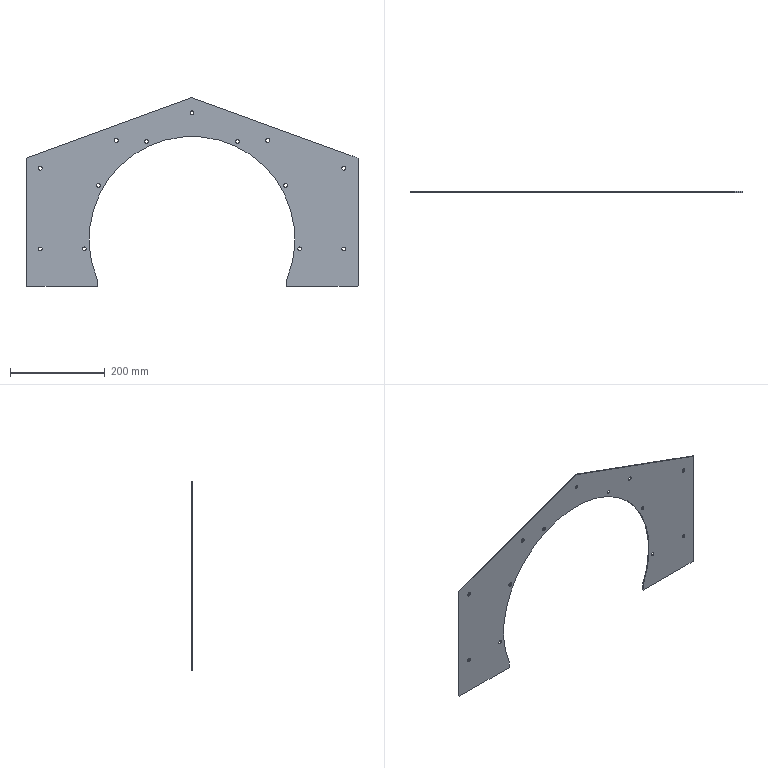Part | NX | features solid 2 | 1 solid | 39 faces | box 700 x 2 x 398 mm | volume 235730 mm3 | cylinder 27 | plane 12 | commonest cylinder face diameters 8 x26 434 x1
STEP:
#1=CARTESIAN_POINT('',(300.,-652.582,589.358));
#2=VERTEX_POINT('',#1);
#3=CARTESIAN_POINT('',(300.,-650.582,589.358));
#4=VERTEX_POINT('',#3);
#5=CARTESIAN_POINT('',(300.,-642.582,589.358));
#6=DIRECTION('',(0.,-1.,0.));
#7=VECTOR('',#6,1000.);
#8=LINE('',#5,#7);
#9=EDGE_CURVE('',#2,#4,#8,.F.);
#10=ORIENTED_EDGE('',*,*,#9,.T.);
#11=CARTESIAN_POINT('',(300.,-650.582,581.358));
#12=VERTEX_POINT('',#11);
#13=CARTESIAN_POINT('',(300.,-650.582,585.358));
#14=DIRECTION('',(0.,1.,0.));
#15=DIRECTION('',(0.,0.,1.));
#16=AXIS2_PLACEMENT_3D('',#13,#14,#15);
#17=CIRCLE('',#16,4.);
#18=EDGE_CURVE('',#4,#12,#17,.T.);
#19=ORIENTED_EDGE('',*,*,#18,.T.);
#20=CARTESIAN_POINT('',(300.,-652.582,581.358));
#21=VERTEX_POINT('',#20);
#22=CARTESIAN_POINT('',(300.,-642.582,581.358));
#23=DIRECTION('',(0.,-1.,0.));
#24=VECTOR('',#23,1000.);
#25=LINE('',#22,#24);
#26=EDGE_CURVE('',#12,#21,#25,.T.);
#27=ORIENTED_EDGE('',*,*,#26,.T.);
#28=CARTESIAN_POINT('',(300.,-652.582,585.358));
#29=DIRECTION('',(0.,-1.,0.));
#30=DIRECTION('',(1.,0.,0.));
#31=AXIS2_PLACEMENT_3D('',#28,#29,#30);
#32=CIRCLE('',#31,4.);
#33=EDGE_CURVE('',#21,#2,#32,.T.);
#34=ORIENTED_EDGE('',*,*,#33,.T.);
#35=EDGE_LOOP('',(#10,#19,#27,#34));
#36=FACE_BOUND('',#35,.T.);
#37=CARTESIAN_POINT('',(300.,-642.582,585.358));
#38=DIRECTION('',(0.,-1.,0.));
#39=DIRECTION('',(0.,0.,-1.));
#40=AXIS2_PLACEMENT_3D('',#37,#38,#39);
#41=CYLINDRICAL_SURFACE('',#40,4.);
#42=ADVANCED_FACE('',(#36),#41,.F.);
#43=CARTESIAN_POINT('',(300.,-650.582,419.358));
#44=VERTEX_POINT('',#43);
#45=CARTESIAN_POINT('',(300.,-652.582,419.358));
#46=VERTEX_POINT('',#45);
#47=CARTESIAN_POINT('',(300.,-642.582,419.358));
#48=DIRECTION('',(0.,-1.,0.));
#49=VECTOR('',#48,1000.);
#50=LINE('',#47,#49);
#51=EDGE_CURVE('',#44,#46,#50,.T.);
#52=ORIENTED_EDGE('',*,*,#51,.F.);
#53=CARTESIAN_POINT('',(300.,-650.582,411.358));
#54=VERTEX_POINT('',#53);
#55=CARTESIAN_POINT('',(300.,-650.582,415.358));
#56=DIRECTION('',(0.,1.,0.));
#57=DIRECTION('',(0.,0.,1.));
#58=AXIS2_PLACEMENT_3D('',#55,#56,#57);
#59=CIRCLE('',#58,4.);
#60=EDGE_CURVE('',#44,#54,#59,.T.);
#61=ORIENTED_EDGE('',*,*,#60,.T.);
#62=CARTESIAN_POINT('',(300.,-652.582,411.358));
#63=VERTEX_POINT('',#62);
#64=CARTESIAN_POINT('',(300.,-642.582,411.358));
#65=DIRECTION('',(0.,-1.,0.));
#66=VECTOR('',#65,1000.);
#67=LINE('',#64,#66);
#68=EDGE_CURVE('',#63,#54,#67,.F.);
#69=ORIENTED_EDGE('',*,*,#68,.F.);
#70=CARTESIAN_POINT('',(300.,-652.582,415.358));
#71=DIRECTION('',(0.,-1.,0.));
#72=DIRECTION('',(1.,0.,0.));
#73=AXIS2_PLACEMENT_3D('',#70,#71,#72);
#74=CIRCLE('',#73,4.);
#75=EDGE_CURVE('',#63,#46,#74,.T.);
#76=ORIENTED_EDGE('',*,*,#75,.T.);
#77=EDGE_LOOP('',(#52,#61,#69,#76));
#78=FACE_BOUND('',#77,.T.);
#79=CARTESIAN_POINT('',(300.,-642.582,415.358));
#80=DIRECTION('',(0.,-1.,0.));
#81=DIRECTION('',(0.,0.,-1.));
#82=AXIS2_PLACEMENT_3D('',#79,#80,#81);
#83=CYLINDRICAL_SURFACE('',#82,4.);
#84=ADVANCED_FACE('',(#78),#83,.F.);
#85=CARTESIAN_POINT('',(207.132,-652.582,419.487));
#86=VERTEX_POINT('',#85);
#87=CARTESIAN_POINT('',(207.132,-650.582,419.487));
#88=VERTEX_POINT('',#87);
#89=CARTESIAN_POINT('',(207.132,-642.582,419.487));
#90=DIRECTION('',(0.,-1.,0.));
#91=VECTOR('',#90,1000.);
#92=LINE('',#89,#91);
#93=EDGE_CURVE('',#86,#88,#92,.F.);
#94=ORIENTED_EDGE('',*,*,#93,.T.);
#95=CARTESIAN_POINT('',(207.132,-650.582,411.487));
#96=VERTEX_POINT('',#95);
#97=CARTESIAN_POINT('',(207.132,-650.582,415.487));
#98=DIRECTION('',(0.,1.,0.));
#99=DIRECTION('',(0.,0.,1.));
#100=AXIS2_PLACEMENT_3D('',#97,#98,#99);
#101=CIRCLE('',#100,4.);
#102=EDGE_CURVE('',#88,#96,#101,.T.);
#103=ORIENTED_EDGE('',*,*,#102,.T.);
#104=CARTESIAN_POINT('',(207.132,-652.582,411.487));
#105=VERTEX_POINT('',#104);
#106=CARTESIAN_POINT('',(207.132,-642.582,411.487));
#107=DIRECTION('',(0.,-1.,0.));
#108=VECTOR('',#107,1000.);
#109=LINE('',#106,#108);
#110=EDGE_CURVE('',#96,#105,#109,.T.);
#111=ORIENTED_EDGE('',*,*,#110,.T.);
#112=CARTESIAN_POINT('',(207.132,-652.582,415.487));
#113=DIRECTION('',(0.,-1.,0.));
#114=DIRECTION('',(1.,0.,0.));
#115=AXIS2_PLACEMENT_3D('',#112,#113,#114);
#116=CIRCLE('',#115,4.);
#117=EDGE_CURVE('',#105,#86,#116,.T.);
#118=ORIENTED_EDGE('',*,*,#117,.T.);
#119=EDGE_LOOP('',(#94,#103,#111,#118));
#120=FACE_BOUND('',#119,.T.);
#121=CARTESIAN_POINT('',(207.132,-642.582,415.487));
#122=DIRECTION('',(0.,-1.,0.));
#123=DIRECTION('',(0.,0.,-1.));
#124=AXIS2_PLACEMENT_3D('',#121,#122,#123);
#125=CYLINDRICAL_SURFACE('',#124,4.);
#126=ADVANCED_FACE('',(#120),#125,.F.);
#127=CARTESIAN_POINT('',(177.334,-650.582,553.289));
#128=VERTEX_POINT('',#127);
#129=CARTESIAN_POINT('',(177.334,-652.582,553.289));
#130=VERTEX_POINT('',#129);
#131=CARTESIAN_POINT('',(177.334,-642.582,553.289));
#132=DIRECTION('',(0.,-1.,0.));
#133=VECTOR('',#132,1000.);
#134=LINE('',#131,#133);
#135=EDGE_CURVE('',#128,#130,#134,.T.);
#136=ORIENTED_EDGE('',*,*,#135,.F.);
#137=CARTESIAN_POINT('',(177.334,-650.582,545.289));
#138=VERTEX_POINT('',#137);
#139=CARTESIAN_POINT('',(177.334,-650.582,549.289));
#140=DIRECTION('',(0.,1.,0.));
#141=DIRECTION('',(0.,0.,1.));
#142=AXIS2_PLACEMENT_3D('',#139,#140,#141);
#143=CIRCLE('',#142,4.);
#144=EDGE_CURVE('',#128,#138,#143,.T.);
#145=ORIENTED_EDGE('',*,*,#144,.T.);
#146=CARTESIAN_POINT('',(177.334,-652.582,545.289));
#147=VERTEX_POINT('',#146);
#148=CARTESIAN_POINT('',(177.334,-642.582,545.289));
#149=DIRECTION('',(0.,-1.,0.));
#150=VECTOR('',#149,1000.);
#151=LINE('',#148,#150);
#152=EDGE_CURVE('',#147,#138,#151,.F.);
#153=ORIENTED_EDGE('',*,*,#152,.F.);
#154=CARTESIAN_POINT('',(177.334,-652.582,549.289));
#155=DIRECTION('',(0.,-1.,0.));
#156=DIRECTION('',(1.,0.,0.));
#157=AXIS2_PLACEMENT_3D('',#154,#155,#156);
#158=CIRCLE('',#157,4.);
#159=EDGE_CURVE('',#147,#130,#158,.T.);
#160=ORIENTED_EDGE('',*,*,#159,.T.);
#161=EDGE_LOOP('',(#136,#145,#153,#160));
#162=FACE_BOUND('',#161,.T.);
#163=CARTESIAN_POINT('',(177.334,-642.582,549.289));
#164=DIRECTION('',(0.,-1.,0.));
#165=DIRECTION('',(0.,0.,-1.));
#166=AXIS2_PLACEMENT_3D('',#163,#164,#165);
#167=CYLINDRICAL_SURFACE('',#166,4.);
#168=ADVANCED_FACE('',(#162),#167,.F.);
#169=CARTESIAN_POINT('',(139.748,-650.582,648.215));
#170=VERTEX_POINT('',#169);
#171=CARTESIAN_POINT('',(139.748,-652.582,648.215));
#172=VERTEX_POINT('',#171);
#173=CARTESIAN_POINT('',(139.748,-642.582,648.215));
#174=DIRECTION('',(0.,-1.,0.));
#175=VECTOR('',#174,1000.);
#176=LINE('',#173,#175);
#177=EDGE_CURVE('',#170,#172,#176,.T.);
#178=ORIENTED_EDGE('',*,*,#177,.F.);
#179=CARTESIAN_POINT('',(139.748,-650.582,640.215));
#180=VERTEX_POINT('',#179);
#181=CARTESIAN_POINT('',(139.748,-650.582,644.215));
#182=DIRECTION('',(0.,1.,0.));
#183=DIRECTION('',(0.,0.,1.));
#184=AXIS2_PLACEMENT_3D('',#181,#182,#183);
#185=CIRCLE('',#184,4.);
#186=EDGE_CURVE('',#170,#180,#185,.T.);
#187=ORIENTED_EDGE('',*,*,#186,.T.);
#188=CARTESIAN_POINT('',(139.748,-652.582,640.215));
#189=VERTEX_POINT('',#188);
#190=CARTESIAN_POINT('',(139.748,-642.582,640.215));
#191=DIRECTION('',(0.,-1.,0.));
#192=VECTOR('',#191,1000.);
#193=LINE('',#190,#192);
#194=EDGE_CURVE('',#189,#180,#193,.F.);
#195=ORIENTED_EDGE('',*,*,#194,.F.);
#196=CARTESIAN_POINT('',(139.748,-652.582,644.215));
#197=DIRECTION('',(0.,-1.,0.));
#198=DIRECTION('',(1.,0.,0.));
#199=AXIS2_PLACEMENT_3D('',#196,#197,#198);
#200=CIRCLE('',#199,4.);
#201=EDGE_CURVE('',#189,#172,#200,.T.);
#202=ORIENTED_EDGE('',*,*,#201,.T.);
#203=EDGE_LOOP('',(#178,#187,#195,#202));
#204=FACE_BOUND('',#203,.T.);
#205=CARTESIAN_POINT('',(139.748,-642.582,644.215));
#206=DIRECTION('',(0.,-1.,0.));
#207=DIRECTION('',(0.,0.,-1.));
#208=AXIS2_PLACEMENT_3D('',#205,#206,#207);
#209=CYLINDRICAL_SURFACE('',#208,4.);
#210=ADVANCED_FACE('',(#204),#209,.F.);
#211=CARTESIAN_POINT('',(76.357,-650.582,645.996));
#212=VERTEX_POINT('',#211);
#213=CARTESIAN_POINT('',(76.357,-652.582,645.996));
#214=VERTEX_POINT('',#213);
#215=CARTESIAN_POINT('',(76.357,-642.582,645.996));
#216=DIRECTION('',(0.,-1.,0.));
#217=VECTOR('',#216,1000.);
#218=LINE('',#215,#217);
#219=EDGE_CURVE('',#212,#214,#218,.T.);
#220=ORIENTED_EDGE('',*,*,#219,.F.);
#221=CARTESIAN_POINT('',(76.357,-650.582,637.996));
#222=VERTEX_POINT('',#221);
#223=CARTESIAN_POINT('',(76.357,-650.582,641.996));
#224=DIRECTION('',(0.,1.,0.));
#225=DIRECTION('',(0.,0.,1.));
#226=AXIS2_PLACEMENT_3D('',#223,#224,#225);
#227=CIRCLE('',#226,4.);
#228=EDGE_CURVE('',#212,#222,#227,.T.);
#229=ORIENTED_EDGE('',*,*,#228,.T.);
#230=CARTESIAN_POINT('',(76.357,-652.582,637.996));
#231=VERTEX_POINT('',#230);
#232=CARTESIAN_POINT('',(76.357,-642.582,637.996));
#233=DIRECTION('',(0.,-1.,0.));
#234=VECTOR('',#233,1000.);
#235=LINE('',#232,#234);
#236=EDGE_CURVE('',#231,#222,#235,.F.);
#237=ORIENTED_EDGE('',*,*,#236,.F.);
#238=CARTESIAN_POINT('',(76.357,-652.582,641.996));
#239=DIRECTION('',(0.,-1.,0.));
#240=DIRECTION('',(1.,0.,0.));
#241=AXIS2_PLACEMENT_3D('',#238,#239,#240);
#242=CIRCLE('',#241,4.);
#243=EDGE_CURVE('',#231,#214,#242,.T.);
#244=ORIENTED_EDGE('',*,*,#243,.T.);
#245=EDGE_LOOP('',(#220,#229,#237,#244));
#246=FACE_BOUND('',#245,.T.);
#247=CARTESIAN_POINT('',(76.357,-642.582,641.996));
#248=DIRECTION('',(0.,-1.,0.));
#249=DIRECTION('',(0.,0.,-1.));
#250=AXIS2_PLACEMENT_3D('',#247,#248,#249);
#251=CYLINDRICAL_SURFACE('',#250,4.);
#252=ADVANCED_FACE('',(#246),#251,.F.);
#253=CARTESIAN_POINT('',(-20.,-650.582,706.358));
#254=VERTEX_POINT('',#253);
#255=CARTESIAN_POINT('',(-20.,-652.582,706.358));
#256=VERTEX_POINT('',#255);
#257=CARTESIAN_POINT('',(-20.,-642.582,706.358));
#258=DIRECTION('',(0.,-1.,0.));
#259=VECTOR('',#258,1000.);
#260=LINE('',#257,#259);
#261=EDGE_CURVE('',#254,#256,#260,.T.);
#262=ORIENTED_EDGE('',*,*,#261,.F.);
#263=CARTESIAN_POINT('',(-20.,-650.582,698.358));
#264=VERTEX_POINT('',#263);
#265=CARTESIAN_POINT('',(-20.,-650.582,702.358));
#266=DIRECTION('',(0.,1.,0.));
#267=DIRECTION('',(0.,0.,1.));
#268=AXIS2_PLACEMENT_3D('',#265,#266,#267);
#269=CIRCLE('',#268,4.);
#270=EDGE_CURVE('',#254,#264,#269,.T.);
#271=ORIENTED_EDGE('',*,*,#270,.T.);
#272=CARTESIAN_POINT('',(-20.,-652.582,698.358));
#273=VERTEX_POINT('',#272);
#274=CARTESIAN_POINT('',(-20.,-642.582,698.358));
#275=DIRECTION('',(0.,-1.,0.));
#276=VECTOR('',#275,1000.);
#277=LINE('',#274,#276);
#278=EDGE_CURVE('',#273,#264,#277,.F.);
#279=ORIENTED_EDGE('',*,*,#278,.F.);
#280=CARTESIAN_POINT('',(-20.,-652.582,702.358));
#281=DIRECTION('',(0.,-1.,0.));
#282=DIRECTION('',(1.,0.,0.));
#283=AXIS2_PLACEMENT_3D('',#280,#281,#282);
#284=CIRCLE('',#283,4.);
#285=EDGE_CURVE('',#273,#256,#284,.T.);
#286=ORIENTED_EDGE('',*,*,#285,.T.);
#287=EDGE_LOOP('',(#262,#271,#279,#286));
#288=FACE_BOUND('',#287,.T.);
#289=CARTESIAN_POINT('',(-20.,-642.582,702.358));
#290=DIRECTION('',(0.,-1.,0.));
#291=DIRECTION('',(0.,0.,-1.));
#292=AXIS2_PLACEMENT_3D('',#289,#290,#291);
#293=CYLINDRICAL_SURFACE('',#292,4.);
#294=ADVANCED_FACE('',(#288),#293,.F.);
#295=CARTESIAN_POINT('',(-179.748,-650.582,648.215));
#296=VERTEX_POINT('',#295);
#297=CARTESIAN_POINT('',(-179.748,-652.582,648.215));
#298=VERTEX_POINT('',#297);
#299=CARTESIAN_POINT('',(-179.748,-642.582,648.215));
#300=DIRECTION('',(0.,-1.,0.));
#301=VECTOR('',#300,1000.);
#302=LINE('',#299,#301);
#303=EDGE_CURVE('',#296,#298,#302,.T.);
#304=ORIENTED_EDGE('',*,*,#303,.F.);
#305=CARTESIAN_POINT('',(-179.748,-650.582,640.215));
#306=VERTEX_POINT('',#305);
#307=CARTESIAN_POINT('',(-179.748,-650.582,644.215));
#308=DIRECTION('',(0.,1.,0.));
#309=DIRECTION('',(0.,0.,1.));
#310=AXIS2_PLACEMENT_3D('',#307,#308,#309);
#311=CIRCLE('',#310,4.);
#312=EDGE_CURVE('',#296,#306,#311,.T.);
#313=ORIENTED_EDGE('',*,*,#312,.T.);
#314=CARTESIAN_POINT('',(-179.748,-652.582,640.215));
#315=VERTEX_POINT('',#314);
#316=CARTESIAN_POINT('',(-179.748,-642.582,640.215));
#317=DIRECTION('',(0.,-1.,0.));
#318=VECTOR('',#317,1000.);
#319=LINE('',#316,#318);
#320=EDGE_CURVE('',#315,#306,#319,.F.);
#321=ORIENTED_EDGE('',*,*,#320,.F.);
#322=CARTESIAN_POINT('',(-179.748,-652.582,644.215));
#323=DIRECTION('',(0.,-1.,0.));
#324=DIRECTION('',(1.,0.,0.));
#325=AXIS2_PLACEMENT_3D('',#322,#323,#324);
#326=CIRCLE('',#325,4.);
#327=EDGE_CURVE('',#315,#298,#326,.T.);
#328=ORIENTED_EDGE('',*,*,#327,.T.);
#329=EDGE_LOOP('',(#304,#313,#321,#328));
#330=FACE_BOUND('',#329,.T.);
#331=CARTESIAN_POINT('',(-179.748,-642.582,644.215));
#332=DIRECTION('',(0.,-1.,0.));
#333=DIRECTION('',(0.,0.,-1.));
#334=AXIS2_PLACEMENT_3D('',#331,#332,#333);
#335=CYLINDRICAL_SURFACE('',#334,4.);
#336=ADVANCED_FACE('',(#330),#335,.F.);
#337=CARTESIAN_POINT('',(-116.357,-650.582,645.996));
#338=VERTEX_POINT('',#337);
#339=CARTESIAN_POINT('',(-116.357,-652.582,645.996));
#340=VERTEX_POINT('',#339);
#341=CARTESIAN_POINT('',(-116.357,-642.582,645.996));
#342=DIRECTION('',(0.,-1.,0.));
#343=VECTOR('',#342,1000.);
#344=LINE('',#341,#343);
#345=EDGE_CURVE('',#338,#340,#344,.T.);
#346=ORIENTED_EDGE('',*,*,#345,.F.);
#347=CARTESIAN_POINT('',(-116.357,-650.582,637.996));
#348=VERTEX_POINT('',#347);
#349=CARTESIAN_POINT('',(-116.357,-650.582,641.996));
#350=DIRECTION('',(0.,1.,0.));
#351=DIRECTION('',(0.,0.,1.));
#352=AXIS2_PLACEMENT_3D('',#349,#350,#351);
#353=CIRCLE('',#352,4.);
#354=EDGE_CURVE('',#338,#348,#353,.T.);
#355=ORIENTED_EDGE('',*,*,#354,.T.);
#356=CARTESIAN_POINT('',(-116.357,-652.582,637.996));
#357=VERTEX_POINT('',#356);
#358=CARTESIAN_POINT('',(-116.357,-642.582,637.996));
#359=DIRECTION('',(0.,-1.,0.));
#360=VECTOR('',#359,1000.);
#361=LINE('',#358,#360);
#362=EDGE_CURVE('',#357,#348,#361,.F.);
#363=ORIENTED_EDGE('',*,*,#362,.F.);
#364=CARTESIAN_POINT('',(-116.357,-652.582,641.996));
#365=DIRECTION('',(0.,-1.,0.));
#366=DIRECTION('',(1.,0.,0.));
#367=AXIS2_PLACEMENT_3D('',#364,#365,#366);
#368=CIRCLE('',#367,4.);
#369=EDGE_CURVE('',#357,#340,#368,.T.);
#370=ORIENTED_EDGE('',*,*,#369,.T.);
#371=EDGE_LOOP('',(#346,#355,#363,#370));
#372=FACE_BOUND('',#371,.T.);
#373=CARTESIAN_POINT('',(-116.357,-642.582,641.996));
#374=DIRECTION('',(0.,-1.,0.));
#375=DIRECTION('',(0.,0.,-1.));
#376=AXIS2_PLACEMENT_3D('',#373,#374,#375);
#377=CYLINDRICAL_SURFACE('',#376,4.);
#378=ADVANCED_FACE('',(#372),#377,.F.);
#379=CARTESIAN_POINT('',(-217.334,-650.582,553.289));
#380=VERTEX_POINT('',#379);
#381=CARTESIAN_POINT('',(-217.334,-652.582,553.289));
#382=VERTEX_POINT('',#381);
#383=CARTESIAN_POINT('',(-217.334,-642.582,553.289));
#384=DIRECTION('',(0.,-1.,0.));
#385=VECTOR('',#384,1000.);
#386=LINE('',#383,#385);
#387=EDGE_CURVE('',#380,#382,#386,.T.);
#388=ORIENTED_EDGE('',*,*,#387,.F.);
#389=CARTESIAN_POINT('',(-217.334,-650.582,545.289));
#390=VERTEX_POINT('',#389);
#391=CARTESIAN_POINT('',(-217.334,-650.582,549.289));
#392=DIRECTION('',(0.,1.,0.));
#393=DIRECTION('',(0.,0.,1.));
#394=AXIS2_PLACEMENT_3D('',#391,#392,#393);
#395=CIRCLE('',#394,4.);
#396=EDGE_CURVE('',#380,#390,#395,.T.);
#397=ORIENTED_EDGE('',*,*,#396,.T.);
#398=CARTESIAN_POINT('',(-217.334,-652.582,545.289));
#399=VERTEX_POINT('',#398);
#400=CARTESIAN_POINT('',(-217.334,-642.582,545.289));
#401=DIRECTION('',(0.,-1.,0.));
#402=VECTOR('',#401,1000.);
#403=LINE('',#400,#402);
#404=EDGE_CURVE('',#399,#390,#403,.F.);
#405=ORIENTED_EDGE('',*,*,#404,.F.);
#406=CARTESIAN_POINT('',(-217.334,-652.582,549.289));
#407=DIRECTION('',(0.,-1.,0.));
#408=DIRECTION('',(1.,0.,0.));
#409=AXIS2_PLACEMENT_3D('',#406,#407,#408);
#410=CIRCLE('',#409,4.);
#411=EDGE_CURVE('',#399,#382,#410,.T.);
#412=ORIENTED_EDGE('',*,*,#411,.T.);
#413=EDGE_LOOP('',(#388,#397,#405,#412));
#414=FACE_BOUND('',#413,.T.);
#415=CARTESIAN_POINT('',(-217.334,-642.582,549.289));
#416=DIRECTION('',(0.,-1.,0.));
#417=DIRECTION('',(0.,0.,-1.));
#418=AXIS2_PLACEMENT_3D('',#415,#416,#417);
#419=CYLINDRICAL_SURFACE('',#418,4.);
#420=ADVANCED_FACE('',(#414),#419,.F.);
#421=CARTESIAN_POINT('',(-247.132,-652.582,419.487));
#422=VERTEX_POINT('',#421);
#423=CARTESIAN_POINT('',(-247.132,-650.582,419.487));
#424=VERTEX_POINT('',#423);
#425=CARTESIAN_POINT('',(-247.132,-642.582,419.487));
#426=DIRECTION('',(0.,-1.,0.));
#427=VECTOR('',#426,1000.);
#428=LINE('',#425,#427);
#429=EDGE_CURVE('',#422,#424,#428,.F.);
#430=ORIENTED_EDGE('',*,*,#429,.T.);
#431=CARTESIAN_POINT('',(-247.132,-650.582,411.487));
#432=VERTEX_POINT('',#431);
#433=CARTESIAN_POINT('',(-247.132,-650.582,415.487));
#434=DIRECTION('',(0.,1.,0.));
#435=DIRECTION('',(0.,0.,1.));
#436=AXIS2_PLACEMENT_3D('',#433,#434,#435);
#437=CIRCLE('',#436,4.);
#438=EDGE_CURVE('',#424,#432,#437,.T.);
#439=ORIENTED_EDGE('',*,*,#438,.T.);
#440=CARTESIAN_POINT('',(-247.132,-652.582,411.487));
#441=VERTEX_POINT('',#440);
#442=CARTESIAN_POINT('',(-247.132,-642.582,411.487));
#443=DIRECTION('',(0.,-1.,0.));
#444=VECTOR('',#443,1000.);
#445=LINE('',#442,#444);
#446=EDGE_CURVE('',#432,#441,#445,.T.);
#447=ORIENTED_EDGE('',*,*,#446,.T.);
#448=CARTESIAN_POINT('',(-247.132,-652.582,415.487));
#449=DIRECTION('',(0.,-1.,0.));
#450=DIRECTION('',(1.,0.,0.));
#451=AXIS2_PLACEMENT_3D('',#448,#449,#450);
#452=CIRCLE('',#451,4.);
#453=EDGE_CURVE('',#441,#422,#452,.T.);
#454=ORIENTED_EDGE('',*,*,#453,.T.);
#455=EDGE_LOOP('',(#430,#439,#447,#454));
#456=FACE_BOUND('',#455,.T.);
#457=CARTESIAN_POINT('',(-247.132,-642.582,415.487));
#458=DIRECTION('',(0.,-1.,0.));
#459=DIRECTION('',(0.,0.,-1.));
#460=AXIS2_PLACEMENT_3D('',#457,#458,#459);
#461=CYLINDRICAL_SURFACE('',#460,4.);
#462=ADVANCED_FACE('',(#456),#461,.F.);
#463=CARTESIAN_POINT('',(-340.,-650.582,419.358));
#464=VERTEX_POINT('',#463);
#465=CARTESIAN_POINT('',(-340.,-652.582,419.358));
#466=VERTEX_POINT('',#465);
#467=CARTESIAN_POINT('',(-340.,-642.582,419.358));
#468=DIRECTION('',(0.,-1.,0.));
#469=VECTOR('',#468,1000.);
#470=LINE('',#467,#469);
#471=EDGE_CURVE('',#464,#466,#470,.T.);
#472=ORIENTED_EDGE('',*,*,#471,.F.);
#473=CARTESIAN_POINT('',(-340.,-650.582,411.358));
#474=VERTEX_POINT('',#473);
#475=CARTESIAN_POINT('',(-340.,-650.582,415.358));
#476=DIRECTION('',(0.,1.,0.));
#477=DIRECTION('',(0.,0.,1.));
#478=AXIS2_PLACEMENT_3D('',#475,#476,#477);
#479=CIRCLE('',#478,4.);
#480=EDGE_CURVE('',#464,#474,#479,.T.);
#481=ORIENTED_EDGE('',*,*,#480,.T.);
#482=CARTESIAN_POINT('',(-340.,-652.582,411.358));
#483=VERTEX_POINT('',#482);
#484=CARTESIAN_POINT('',(-340.,-642.582,411.358));
#485=DIRECTION('',(0.,-1.,0.));
#486=VECTOR('',#485,1000.);
#487=LINE('',#484,#486);
#488=EDGE_CURVE('',#483,#474,#487,.F.);
#489=ORIENTED_EDGE('',*,*,#488,.F.);
#490=CARTESIAN_POINT('',(-340.,-652.582,415.358));
#491=DIRECTION('',(0.,-1.,0.));
#492=DIRECTION('',(1.,0.,0.));
#493=AXIS2_PLACEMENT_3D('',#490,#491,#492);
#494=CIRCLE('',#493,4.);
#495=EDGE_CURVE('',#483,#466,#494,.T.);
#496=ORIENTED_EDGE('',*,*,#495,.T.);
#497=EDGE_LOOP('',(#472,#481,#489,#496));
#498=FACE_BOUND('',#497,.T.);
#499=CARTESIAN_POINT('',(-340.,-642.582,415.358));
#500=DIRECTION('',(0.,-1.,0.));
#501=DIRECTION('',(0.,0.,-1.));
#502=AXIS2_PLACEMENT_3D('',#499,#500,#501);
#503=CYLINDRICAL_SURFACE('',#502,4.);
#504=ADVANCED_FACE('',(#498),#503,.F.);
#505=CARTESIAN_POINT('',(-340.,-650.582,589.358));
#506=VERTEX_POINT('',#505);
#507=CARTESIAN_POINT('',(-340.,-652.582,589.358));
#508=VERTEX_POINT('',#507);
#509=CARTESIAN_POINT('',(-340.,-642.582,589.358));
#510=DIRECTION('',(0.,-1.,0.));
#511=VECTOR('',#510,1000.);
#512=LINE('',#509,#511);
#513=EDGE_CURVE('',#506,#508,#512,.T.);
#514=ORIENTED_EDGE('',*,*,#513,.F.);
#515=CARTESIAN_POINT('',(-340.,-650.582,581.358));
#516=VERTEX_POINT('',#515);
#517=CARTESIAN_POINT('',(-340.,-650.582,585.358));
#518=DIRECTION('',(0.,1.,0.));
#519=DIRECTION('',(0.,0.,1.));
#520=AXIS2_PLACEMENT_3D('',#517,#518,#519);
#521=CIRCLE('',#520,4.);
#522=EDGE_CURVE('',#506,#516,#521,.T.);
#523=ORIENTED_EDGE('',*,*,#522,.T.);
#524=CARTESIAN_POINT('',(-340.,-652.582,581.358));
#525=VERTEX_POINT('',#524);
#526=CARTESIAN_POINT('',(-340.,-642.582,581.358));
#527=DIRECTION('',(0.,-1.,0.));
#528=VECTOR('',#527,1000.);
#529=LINE('',#526,#528);
#530=EDGE_CURVE('',#525,#516,#529,.F.);
#531=ORIENTED_EDGE('',*,*,#530,.F.);
#532=CARTESIAN_POINT('',(-340.,-652.582,585.358));
#533=DIRECTION('',(0.,-1.,0.));
#534=DIRECTION('',(1.,0.,0.));
#535=AXIS2_PLACEMENT_3D('',#532,#533,#534);
#536=CIRCLE('',#535,4.);
#537=EDGE_CURVE('',#525,#508,#536,.T.);
#538=ORIENTED_EDGE('',*,*,#537,.T.);
#539=EDGE_LOOP('',(#514,#523,#531,#538));
#540=FACE_BOUND('',#539,.T.);
#541=CARTESIAN_POINT('',(-340.,-642.582,585.358));
#542=DIRECTION('',(0.,-1.,0.));
#543=DIRECTION('',(0.,0.,-1.));
#544=AXIS2_PLACEMENT_3D('',#541,#542,#543);
#545=CYLINDRICAL_SURFACE('',#544,4.);
#546=ADVANCED_FACE('',(#540),#545,.F.);
#547=ORIENTED_EDGE('',*,*,#537,.F.);
#548=CARTESIAN_POINT('',(-340.,-652.582,585.358));
#549=DIRECTION('',(0.,-1.,0.));
#550=DIRECTION('',(1.,0.,0.));
#551=AXIS2_PLACEMENT_3D('',#548,#549,#550);
#552=CIRCLE('',#551,4.);
#553=EDGE_CURVE('',#508,#525,#552,.T.);
#554=ORIENTED_EDGE('',*,*,#553,.F.);
#555=EDGE_LOOP('',(#547,#554));
#556=FACE_BOUND('',#555,.T.);
#557=ORIENTED_EDGE('',*,*,#495,.F.);
#558=CARTESIAN_POINT('',(-340.,-652.582,415.358));
#559=DIRECTION('',(0.,-1.,0.));
#560=DIRECTION('',(1.,0.,0.));
#561=AXIS2_PLACEMENT_3D('',#558,#559,#560);
#562=CIRCLE('',#561,4.);
#563=EDGE_CURVE('',#466,#483,#562,.T.);
#564=ORIENTED_EDGE('',*,*,#563,.F.);
#565=EDGE_LOOP('',(#557,#564));
#566=FACE_BOUND('',#565,.T.);
#567=ORIENTED_EDGE('',*,*,#453,.F.);
#568=CARTESIAN_POINT('',(-247.132,-652.582,415.487));
#569=DIRECTION('',(0.,-1.,0.));
#570=DIRECTION('',(1.,0.,0.));
#571=AXIS2_PLACEMENT_3D('',#568,#569,#570);
#572=CIRCLE('',#571,4.);
#573=EDGE_CURVE('',#422,#441,#572,.T.);
#574=ORIENTED_EDGE('',*,*,#573,.F.);
#575=EDGE_LOOP('',(#567,#574));
#576=FACE_BOUND('',#575,.T.);
#577=ORIENTED_EDGE('',*,*,#411,.F.);
#578=CARTESIAN_POINT('',(-217.334,-652.582,549.289));
#579=DIRECTION('',(0.,-1.,0.));
#580=DIRECTION('',(1.,0.,0.));
#581=AXIS2_PLACEMENT_3D('',#578,#579,#580);
#582=CIRCLE('',#581,4.);
#583=EDGE_CURVE('',#382,#399,#582,.T.);
#584=ORIENTED_EDGE('',*,*,#583,.F.);
#585=EDGE_LOOP('',(#577,#584));
#586=FACE_BOUND('',#585,.T.);
#587=ORIENTED_EDGE('',*,*,#369,.F.);
#588=CARTESIAN_POINT('',(-116.357,-652.582,641.996));
#589=DIRECTION('',(0.,-1.,0.));
#590=DIRECTION('',(1.,0.,0.));
#591=AXIS2_PLACEMENT_3D('',#588,#589,#590);
#592=CIRCLE('',#591,4.);
#593=EDGE_CURVE('',#340,#357,#592,.T.);
#594=ORIENTED_EDGE('',*,*,#593,.F.);
#595=EDGE_LOOP('',(#587,#594));
#596=FACE_BOUND('',#595,.T.);
#597=ORIENTED_EDGE('',*,*,#327,.F.);
#598=CARTESIAN_POINT('',(-179.748,-652.582,644.215));
#599=DIRECTION('',(0.,-1.,0.));
#600=DIRECTION('',(1.,0.,0.));
#601=AXIS2_PLACEMENT_3D('',#598,#599,#600);
#602=CIRCLE('',#601,4.);
#603=EDGE_CURVE('',#298,#315,#602,.T.);
#604=ORIENTED_EDGE('',*,*,#603,.F.);
#605=EDGE_LOOP('',(#597,#604));
#606=FACE_BOUND('',#605,.T.);
#607=ORIENTED_EDGE('',*,*,#285,.F.);
#608=CARTESIAN_POINT('',(-20.,-652.582,702.358));
#609=DIRECTION('',(0.,-1.,0.));
#610=DIRECTION('',(1.,0.,0.));
#611=AXIS2_PLACEMENT_3D('',#608,#609,#610);
#612=CIRCLE('',#611,4.);
#613=EDGE_CURVE('',#256,#273,#612,.T.);
#614=ORIENTED_EDGE('',*,*,#613,.F.);
#615=EDGE_LOOP('',(#607,#614));
#616=FACE_BOUND('',#615,.T.);
#617=ORIENTED_EDGE('',*,*,#243,.F.);
#618=CARTESIAN_POINT('',(76.357,-652.582,641.996));
#619=DIRECTION('',(0.,-1.,0.));
#620=DIRECTION('',(1.,0.,0.));
#621=AXIS2_PLACEMENT_3D('',#618,#619,#620);
#622=CIRCLE('',#621,4.);
#623=EDGE_CURVE('',#214,#231,#622,.T.);
#624=ORIENTED_EDGE('',*,*,#623,.F.);
#625=EDGE_LOOP('',(#617,#624));
#626=FACE_BOUND('',#625,.T.);
#627=ORIENTED_EDGE('',*,*,#201,.F.);
#628=CARTESIAN_POINT('',(139.748,-652.582,644.215));
#629=DIRECTION('',(0.,-1.,0.));
#630=DIRECTION('',(1.,0.,0.));
#631=AXIS2_PLACEMENT_3D('',#628,#629,#630);
#632=CIRCLE('',#631,4.);
#633=EDGE_CURVE('',#172,#189,#632,.T.);
#634=ORIENTED_EDGE('',*,*,#633,.F.);
#635=EDGE_LOOP('',(#627,#634));
#636=FACE_BOUND('',#635,.T.);
#637=ORIENTED_EDGE('',*,*,#159,.F.);
#638=CARTESIAN_POINT('',(177.334,-652.582,549.289));
#639=DIRECTION('',(0.,-1.,0.));
#640=DIRECTION('',(1.,0.,0.));
#641=AXIS2_PLACEMENT_3D('',#638,#639,#640);
#642=CIRCLE('',#641,4.);
#643=EDGE_CURVE('',#130,#147,#642,.T.);
#644=ORIENTED_EDGE('',*,*,#643,.F.);
#645=EDGE_LOOP('',(#637,#644));
#646=FACE_BOUND('',#645,.T.);
#647=ORIENTED_EDGE('',*,*,#117,.F.);
#648=CARTESIAN_POINT('',(207.132,-652.582,415.487));
#649=DIRECTION('',(0.,-1.,0.));
#650=DIRECTION('',(1.,0.,0.));
#651=AXIS2_PLACEMENT_3D('',#648,#649,#650);
#652=CIRCLE('',#651,4.);
#653=EDGE_CURVE('',#86,#105,#652,.T.);
#654=ORIENTED_EDGE('',*,*,#653,.F.);
#655=EDGE_LOOP('',(#647,#654));
#656=FACE_BOUND('',#655,.T.);
#657=ORIENTED_EDGE('',*,*,#75,.F.);
#658=CARTESIAN_POINT('',(300.,-652.582,415.358));
#659=DIRECTION('',(0.,-1.,0.));
#660=DIRECTION('',(1.,0.,0.));
#661=AXIS2_PLACEMENT_3D('',#658,#659,#660);
#662=CIRCLE('',#661,4.);
#663=EDGE_CURVE('',#46,#63,#662,.T.);
#664=ORIENTED_EDGE('',*,*,#663,.F.);
#665=EDGE_LOOP('',(#657,#664));
#666=FACE_BOUND('',#665,.T.);
#667=ORIENTED_EDGE('',*,*,#33,.F.);
#668=CARTESIAN_POINT('',(300.,-652.582,585.358));
#669=DIRECTION('',(0.,-1.,0.));
#670=DIRECTION('',(1.,0.,0.));
#671=AXIS2_PLACEMENT_3D('',#668,#669,#670);
#672=CIRCLE('',#671,4.);
#673=EDGE_CURVE('',#2,#21,#672,.T.);
#674=ORIENTED_EDGE('',*,*,#673,.F.);
#675=EDGE_LOOP('',(#667,#674));
#676=FACE_BOUND('',#675,.T.);
#677=CARTESIAN_POINT('',(330.,-652.582,338.358));
#678=VERTEX_POINT('',#677);
#679=CARTESIAN_POINT('',(330.,-652.582,606.969));
#680=VERTEX_POINT('',#679);
#681=CARTESIAN_POINT('',(330.,-652.582,606.969));
#682=DIRECTION('',(0.,0.,1.));
#683=VECTOR('',#682,1000.);
#684=LINE('',#681,#683);
#685=EDGE_CURVE('',#678,#680,#684,.T.);
#686=ORIENTED_EDGE('',*,*,#685,.T.);
#687=CARTESIAN_POINT('',(-20.,-652.582,734.358));
#688=VERTEX_POINT('',#687);
#689=CARTESIAN_POINT('',(330.,-652.582,606.969));
#690=DIRECTION('',(-0.9397,0.,0.342));
#691=VECTOR('',#690,1000.);
#692=LINE('',#689,#691);
#693=EDGE_CURVE('',#680,#688,#692,.T.);
#694=ORIENTED_EDGE('',*,*,#693,.T.);
#695=CARTESIAN_POINT('',(-370.,-652.582,606.969));
#696=VERTEX_POINT('',#695);
#697=CARTESIAN_POINT('',(-370.,-652.582,606.969));
#698=DIRECTION('',(-0.9397,0.,-0.342));
#699=VECTOR('',#698,1000.);
#700=LINE('',#697,#699);
#701=EDGE_CURVE('',#688,#696,#700,.T.);
#702=ORIENTED_EDGE('',*,*,#701,.T.);
#703=CARTESIAN_POINT('',(-370.,-652.582,338.358));
#704=VERTEX_POINT('',#703);
#705=CARTESIAN_POINT('',(-370.,-652.582,606.969));
#706=DIRECTION('',(0.,0.,-1.));
#707=VECTOR('',#706,1000.);
#708=LINE('',#705,#707);
#709=EDGE_CURVE('',#696,#704,#708,.T.);
#710=ORIENTED_EDGE('',*,*,#709,.T.);
#711=CARTESIAN_POINT('',(-368.,-652.582,336.358));
#712=VERTEX_POINT('',#711);
#713=CARTESIAN_POINT('',(-370.,-652.582,338.358));
#714=DIRECTION('',(0.7071,0.,-0.7071));
#715=VECTOR('',#714,1000.);
#716=LINE('',#713,#715);
#717=EDGE_CURVE('',#704,#712,#716,.T.);
#718=ORIENTED_EDGE('',*,*,#717,.T.);
#719=CARTESIAN_POINT('',(-220.,-652.582,336.358));
#720=VERTEX_POINT('',#719);
#721=CARTESIAN_POINT('',(-368.,-652.582,336.358));
#722=DIRECTION('',(1.,0.,0.));
#723=VECTOR('',#722,1000.);
#724=LINE('',#721,#723);
#725=EDGE_CURVE('',#712,#720,#724,.T.);
#726=ORIENTED_EDGE('',*,*,#725,.T.);
#727=CARTESIAN_POINT('',(-220.,-652.582,351.162));
#728=VERTEX_POINT('',#727);
#729=CARTESIAN_POINT('',(-220.,-652.582,351.162));
#730=DIRECTION('',(0.,0.,1.));
#731=VECTOR('',#730,1000.);
#732=LINE('',#729,#731);
#733=EDGE_CURVE('',#720,#728,#732,.T.);
#734=ORIENTED_EDGE('',*,*,#733,.T.);
#735=CARTESIAN_POINT('',(180.,-652.582,351.162));
#736=VERTEX_POINT('',#735);
#737=CARTESIAN_POINT('',(-20.,-652.582,435.358));
#738=DIRECTION('',(0.,1.,0.));
#739=DIRECTION('',(0.,0.,-1.));
#740=AXIS2_PLACEMENT_3D('',#737,#738,#739);
#741=CIRCLE('',#740,217.);
#742=EDGE_CURVE('',#728,#736,#741,.T.);
#743=ORIENTED_EDGE('',*,*,#742,.T.);
#744=CARTESIAN_POINT('',(180.,-652.582,336.358));
#745=VERTEX_POINT('',#744);
#746=CARTESIAN_POINT('',(180.,-652.582,351.162));
#747=DIRECTION('',(0.,0.,-1.));
#748=VECTOR('',#747,1000.);
#749=LINE('',#746,#748);
#750=EDGE_CURVE('',#736,#745,#749,.T.);
#751=ORIENTED_EDGE('',*,*,#750,.T.);
#752=CARTESIAN_POINT('',(328.,-652.582,336.358));
#753=VERTEX_POINT('',#752);
#754=CARTESIAN_POINT('',(328.,-652.582,336.358));
#755=DIRECTION('',(1.,0.,0.));
#756=VECTOR('',#755,1000.);
#757=LINE('',#754,#756);
#758=EDGE_CURVE('',#745,#753,#757,.T.);
#759=ORIENTED_EDGE('',*,*,#758,.T.);
#760=CARTESIAN_POINT('',(328.,-652.582,336.358));
#761=DIRECTION('',(0.7071,0.,0.7071));
#762=VECTOR('',#761,1000.);
#763=LINE('',#760,#762);
#764=EDGE_CURVE('',#753,#678,#763,.T.);
#765=ORIENTED_EDGE('',*,*,#764,.T.);
#766=EDGE_LOOP('',(#686,#694,#702,#710,#718,#726,#734,#743,#751,#759,#765));
#767=FACE_BOUND('',#766,.T.);
#768=CARTESIAN_POINT('',(-20.,-652.582,435.358));
#769=DIRECTION('',(0.,1.,0.));
#770=DIRECTION('',(1.,0.,0.));
#771=AXIS2_PLACEMENT_3D('',#768,#769,#770);
#772=PLANE('',#771);
#773=ADVANCED_FACE('',(#556,#566,#576,#586,#596,#606,#616,#626,#636,#646,#656,#666,#676,#767),#772,.F.);
#774=CARTESIAN_POINT('',(-340.,-650.582,585.358));
#775=DIRECTION('',(0.,1.,0.));
#776=DIRECTION('',(0.,0.,1.));
#777=AXIS2_PLACEMENT_3D('',#774,#775,#776);
#778=CIRCLE('',#777,4.);
#779=EDGE_CURVE('',#516,#506,#778,.T.);
#780=ORIENTED_EDGE('',*,*,#779,.F.);
#781=ORIENTED_EDGE('',*,*,#522,.F.);
#782=EDGE_LOOP('',(#780,#781));
#783=FACE_BOUND('',#782,.T.);
#784=CARTESIAN_POINT('',(-340.,-650.582,415.358));
#785=DIRECTION('',(0.,1.,0.));
#786=DIRECTION('',(0.,0.,1.));
#787=AXIS2_PLACEMENT_3D('',#784,#785,#786);
#788=CIRCLE('',#787,4.);
#789=EDGE_CURVE('',#474,#464,#788,.T.);
#790=ORIENTED_EDGE('',*,*,#789,.F.);
#791=ORIENTED_EDGE('',*,*,#480,.F.);
#792=EDGE_LOOP('',(#790,#791));
#793=FACE_BOUND('',#792,.T.);
#794=CARTESIAN_POINT('',(-247.132,-650.582,415.487));
#795=DIRECTION('',(0.,1.,0.));
#796=DIRECTION('',(0.,0.,1.));
#797=AXIS2_PLACEMENT_3D('',#794,#795,#796);
#798=CIRCLE('',#797,4.);
#799=EDGE_CURVE('',#432,#424,#798,.T.);
#800=ORIENTED_EDGE('',*,*,#799,.F.);
#801=ORIENTED_EDGE('',*,*,#438,.F.);
#802=EDGE_LOOP('',(#800,#801));
#803=FACE_BOUND('',#802,.T.);
#804=CARTESIAN_POINT('',(-217.334,-650.582,549.289));
#805=DIRECTION('',(0.,1.,0.));
#806=DIRECTION('',(0.,0.,1.));
#807=AXIS2_PLACEMENT_3D('',#804,#805,#806);
#808=CIRCLE('',#807,4.);
#809=EDGE_CURVE('',#390,#380,#808,.T.);
#810=ORIENTED_EDGE('',*,*,#809,.F.);
#811=ORIENTED_EDGE('',*,*,#396,.F.);
#812=EDGE_LOOP('',(#810,#811));
#813=FACE_BOUND('',#812,.T.);
#814=CARTESIAN_POINT('',(-116.357,-650.582,641.996));
#815=DIRECTION('',(0.,1.,0.));
#816=DIRECTION('',(0.,0.,1.));
#817=AXIS2_PLACEMENT_3D('',#814,#815,#816);
#818=CIRCLE('',#817,4.);
#819=EDGE_CURVE('',#348,#338,#818,.T.);
#820=ORIENTED_EDGE('',*,*,#819,.F.);
#821=ORIENTED_EDGE('',*,*,#354,.F.);
#822=EDGE_LOOP('',(#820,#821));
#823=FACE_BOUND('',#822,.T.);
#824=CARTESIAN_POINT('',(-179.748,-650.582,644.215));
#825=DIRECTION('',(0.,1.,0.));
#826=DIRECTION('',(0.,0.,1.));
#827=AXIS2_PLACEMENT_3D('',#824,#825,#826);
#828=CIRCLE('',#827,4.);
#829=EDGE_CURVE('',#306,#296,#828,.T.);
#830=ORIENTED_EDGE('',*,*,#829,.F.);
#831=ORIENTED_EDGE('',*,*,#312,.F.);
#832=EDGE_LOOP('',(#830,#831));
#833=FACE_BOUND('',#832,.T.);
#834=CARTESIAN_POINT('',(-20.,-650.582,702.358));
#835=DIRECTION('',(0.,1.,0.));
#836=DIRECTION('',(0.,0.,1.));
#837=AXIS2_PLACEMENT_3D('',#834,#835,#836);
#838=CIRCLE('',#837,4.);
#839=EDGE_CURVE('',#264,#254,#838,.T.);
#840=ORIENTED_EDGE('',*,*,#839,.F.);
#841=ORIENTED_EDGE('',*,*,#270,.F.);
#842=EDGE_LOOP('',(#840,#841));
#843=FACE_BOUND('',#842,.T.);
#844=CARTESIAN_POINT('',(76.357,-650.582,641.996));
#845=DIRECTION('',(0.,1.,0.));
#846=DIRECTION('',(0.,0.,1.));
#847=AXIS2_PLACEMENT_3D('',#844,#845,#846);
#848=CIRCLE('',#847,4.);
#849=EDGE_CURVE('',#222,#212,#848,.T.);
#850=ORIENTED_EDGE('',*,*,#849,.F.);
#851=ORIENTED_EDGE('',*,*,#228,.F.);
#852=EDGE_LOOP('',(#850,#851));
#853=FACE_BOUND('',#852,.T.);
#854=CARTESIAN_POINT('',(139.748,-650.582,644.215));
#855=DIRECTION('',(0.,1.,0.));
#856=DIRECTION('',(0.,0.,1.));
#857=AXIS2_PLACEMENT_3D('',#854,#855,#856);
#858=CIRCLE('',#857,4.);
#859=EDGE_CURVE('',#180,#170,#858,.T.);
#860=ORIENTED_EDGE('',*,*,#859,.F.);
#861=ORIENTED_EDGE('',*,*,#186,.F.);
#862=EDGE_LOOP('',(#860,#861));
#863=FACE_BOUND('',#862,.T.);
#864=CARTESIAN_POINT('',(177.334,-650.582,549.289));
#865=DIRECTION('',(0.,1.,0.));
#866=DIRECTION('',(0.,0.,1.));
#867=AXIS2_PLACEMENT_3D('',#864,#865,#866);
#868=CIRCLE('',#867,4.);
#869=EDGE_CURVE('',#138,#128,#868,.T.);
#870=ORIENTED_EDGE('',*,*,#869,.F.);
#871=ORIENTED_EDGE('',*,*,#144,.F.);
#872=EDGE_LOOP('',(#870,#871));
#873=FACE_BOUND('',#872,.T.);
#874=CARTESIAN_POINT('',(207.132,-650.582,415.487));
#875=DIRECTION('',(0.,1.,0.));
#876=DIRECTION('',(0.,0.,1.));
#877=AXIS2_PLACEMENT_3D('',#874,#875,#876);
#878=CIRCLE('',#877,4.);
#879=EDGE_CURVE('',#96,#88,#878,.T.);
#880=ORIENTED_EDGE('',*,*,#879,.F.);
#881=ORIENTED_EDGE('',*,*,#102,.F.);
#882=EDGE_LOOP('',(#880,#881));
#883=FACE_BOUND('',#882,.T.);
#884=CARTESIAN_POINT('',(300.,-650.582,415.358));
#885=DIRECTION('',(0.,1.,0.));
#886=DIRECTION('',(0.,0.,1.));
#887=AXIS2_PLACEMENT_3D('',#884,#885,#886);
#888=CIRCLE('',#887,4.);
#889=EDGE_CURVE('',#54,#44,#888,.T.);
#890=ORIENTED_EDGE('',*,*,#889,.F.);
#891=ORIENTED_EDGE('',*,*,#60,.F.);
#892=EDGE_LOOP('',(#890,#891));
#893=FACE_BOUND('',#892,.T.);
#894=CARTESIAN_POINT('',(300.,-650.582,585.358));
#895=DIRECTION('',(0.,1.,0.));
#896=DIRECTION('',(0.,0.,1.));
#897=AXIS2_PLACEMENT_3D('',#894,#895,#896);
#898=CIRCLE('',#897,4.);
#899=EDGE_CURVE('',#12,#4,#898,.T.);
#900=ORIENTED_EDGE('',*,*,#899,.F.);
#901=ORIENTED_EDGE('',*,*,#18,.F.);
#902=EDGE_LOOP('',(#900,#901));
#903=FACE_BOUND('',#902,.T.);
#904=CARTESIAN_POINT('',(330.,-650.582,338.358));
#905=VERTEX_POINT('',#904);
#906=CARTESIAN_POINT('',(330.,-650.582,606.969));
#907=VERTEX_POINT('',#906);
#908=CARTESIAN_POINT('',(330.,-650.582,606.969));
#909=DIRECTION('',(0.,0.,1.));
#910=VECTOR('',#909,1000.);
#911=LINE('',#908,#910);
#912=EDGE_CURVE('',#905,#907,#911,.T.);
#913=ORIENTED_EDGE('',*,*,#912,.F.);
#914=CARTESIAN_POINT('',(328.,-650.582,336.358));
#915=VERTEX_POINT('',#914);
#916=CARTESIAN_POINT('',(328.,-650.582,336.358));
#917=DIRECTION('',(0.7071,0.,0.7071));
#918=VECTOR('',#917,1000.);
#919=LINE('',#916,#918);
#920=EDGE_CURVE('',#915,#905,#919,.T.);
#921=ORIENTED_EDGE('',*,*,#920,.F.);
#922=CARTESIAN_POINT('',(180.,-650.582,336.358));
#923=VERTEX_POINT('',#922);
#924=CARTESIAN_POINT('',(328.,-650.582,336.358));
#925=DIRECTION('',(1.,0.,0.));
#926=VECTOR('',#925,1000.);
#927=LINE('',#924,#926);
#928=EDGE_CURVE('',#923,#915,#927,.T.);
#929=ORIENTED_EDGE('',*,*,#928,.F.);
#930=CARTESIAN_POINT('',(180.,-650.582,351.162));
#931=VERTEX_POINT('',#930);
#932=CARTESIAN_POINT('',(180.,-650.582,351.162));
#933=DIRECTION('',(0.,0.,-1.));
#934=VECTOR('',#933,1000.);
#935=LINE('',#932,#934);
#936=EDGE_CURVE('',#931,#923,#935,.T.);
#937=ORIENTED_EDGE('',*,*,#936,.F.);
#938=CARTESIAN_POINT('',(-220.,-650.582,351.162));
#939=VERTEX_POINT('',#938);
#940=CARTESIAN_POINT('',(-20.,-650.582,435.358));
#941=DIRECTION('',(0.,1.,0.));
#942=DIRECTION('',(0.,0.,-1.));
#943=AXIS2_PLACEMENT_3D('',#940,#941,#942);
#944=CIRCLE('',#943,217.);
#945=EDGE_CURVE('',#939,#931,#944,.T.);
#946=ORIENTED_EDGE('',*,*,#945,.F.);
#947=CARTESIAN_POINT('',(-220.,-650.582,336.358));
#948=VERTEX_POINT('',#947);
#949=CARTESIAN_POINT('',(-220.,-650.582,351.162));
#950=DIRECTION('',(0.,0.,1.));
#951=VECTOR('',#950,1000.);
#952=LINE('',#949,#951);
#953=EDGE_CURVE('',#948,#939,#952,.T.);
#954=ORIENTED_EDGE('',*,*,#953,.F.);
#955=CARTESIAN_POINT('',(-368.,-650.582,336.358));
#956=VERTEX_POINT('',#955);
#957=CARTESIAN_POINT('',(-368.,-650.582,336.358));
#958=DIRECTION('',(1.,0.,0.));
#959=VECTOR('',#958,1000.);
#960=LINE('',#957,#959);
#961=EDGE_CURVE('',#956,#948,#960,.T.);
#962=ORIENTED_EDGE('',*,*,#961,.F.);
#963=CARTESIAN_POINT('',(-370.,-650.582,338.358));
#964=VERTEX_POINT('',#963);
#965=CARTESIAN_POINT('',(-370.,-650.582,338.358));
#966=DIRECTION('',(0.7071,0.,-0.7071));
#967=VECTOR('',#966,1000.);
#968=LINE('',#965,#967);
#969=EDGE_CURVE('',#964,#956,#968,.T.);
#970=ORIENTED_EDGE('',*,*,#969,.F.);
#971=CARTESIAN_POINT('',(-370.,-650.582,606.969));
#972=VERTEX_POINT('',#971);
#973=CARTESIAN_POINT('',(-370.,-650.582,606.969));
#974=DIRECTION('',(0.,0.,-1.));
#975=VECTOR('',#974,1000.);
#976=LINE('',#973,#975);
#977=EDGE_CURVE('',#972,#964,#976,.T.);
#978=ORIENTED_EDGE('',*,*,#977,.F.);
#979=CARTESIAN_POINT('',(-20.,-650.582,734.358));
#980=VERTEX_POINT('',#979);
#981=CARTESIAN_POINT('',(-370.,-650.582,606.969));
#982=DIRECTION('',(-0.9397,0.,-0.342));
#983=VECTOR('',#982,1000.);
#984=LINE('',#981,#983);
#985=EDGE_CURVE('',#980,#972,#984,.T.);
#986=ORIENTED_EDGE('',*,*,#985,.F.);
#987=CARTESIAN_POINT('',(330.,-650.582,606.969));
#988=DIRECTION('',(-0.9397,0.,0.342));
#989=VECTOR('',#988,1000.);
#990=LINE('',#987,#989);
#991=EDGE_CURVE('',#907,#980,#990,.T.);
#992=ORIENTED_EDGE('',*,*,#991,.F.);
#993=EDGE_LOOP('',(#913,#921,#929,#937,#946,#954,#962,#970,#978,#986,#992));
#994=FACE_BOUND('',#993,.T.);
#995=CARTESIAN_POINT('',(-20.,-650.582,435.358));
#996=DIRECTION('',(0.,1.,0.));
#997=DIRECTION('',(1.,0.,0.));
#998=AXIS2_PLACEMENT_3D('',#995,#996,#997);
#999=PLANE('',#998);
#1000=ADVANCED_FACE('',(#783,#793,#803,#813,#823,#833,#843,#853,#863,#873,#883,#893,#903,#994),#999,.T.);
#1001=ORIENTED_EDGE('',*,*,#764,.F.);
#1002=CARTESIAN_POINT('',(328.,-650.582,336.358));
#1003=DIRECTION('',(0.,-1.,0.));
#1004=VECTOR('',#1003,1000.);
#1005=LINE('',#1002,#1004);
#1006=EDGE_CURVE('',#915,#753,#1005,.T.);
#1007=ORIENTED_EDGE('',*,*,#1006,.F.);
#1008=ORIENTED_EDGE('',*,*,#920,.T.);
#1009=CARTESIAN_POINT('',(330.,-650.582,338.358));
#1010=DIRECTION('',(0.,-1.,0.));
#1011=VECTOR('',#1010,1000.);
#1012=LINE('',#1009,#1011);
#1013=EDGE_CURVE('',#905,#678,#1012,.T.);
#1014=ORIENTED_EDGE('',*,*,#1013,.T.);
#1015=EDGE_LOOP('',(#1001,#1007,#1008,#1014));
#1016=FACE_BOUND('',#1015,.T.);
#1017=CARTESIAN_POINT('',(328.,-650.582,336.358));
#1018=DIRECTION('',(0.7071,0.,-0.7071));
#1019=DIRECTION('',(0.,-1.,0.));
#1020=AXIS2_PLACEMENT_3D('',#1017,#1018,#1019);
#1021=PLANE('',#1020);
#1022=ADVANCED_FACE('',(#1016),#1021,.T.);
#1023=ORIENTED_EDGE('',*,*,#758,.F.);
#1024=CARTESIAN_POINT('',(180.,-650.582,336.358));
#1025=DIRECTION('',(0.,-1.,0.));
#1026=VECTOR('',#1025,1000.);
#1027=LINE('',#1024,#1026);
#1028=EDGE_CURVE('',#923,#745,#1027,.T.);
#1029=ORIENTED_EDGE('',*,*,#1028,.F.);
#1030=ORIENTED_EDGE('',*,*,#928,.T.);
#1031=ORIENTED_EDGE('',*,*,#1006,.T.);
#1032=EDGE_LOOP('',(#1023,#1029,#1030,#1031));
#1033=FACE_BOUND('',#1032,.T.);
#1034=CARTESIAN_POINT('',(328.,-650.582,336.358));
#1035=DIRECTION('',(0.,0.,-1.));
#1036=DIRECTION('',(0.,-1.,0.));
#1037=AXIS2_PLACEMENT_3D('',#1034,#1035,#1036);
#1038=PLANE('',#1037);
#1039=ADVANCED_FACE('',(#1033),#1038,.T.);
#1040=ORIENTED_EDGE('',*,*,#750,.F.);
#1041=CARTESIAN_POINT('',(180.,-650.582,351.162));
#1042=DIRECTION('',(0.,-1.,0.));
#1043=VECTOR('',#1042,1000.);
#1044=LINE('',#1041,#1043);
#1045=EDGE_CURVE('',#931,#736,#1044,.T.);
#1046=ORIENTED_EDGE('',*,*,#1045,.F.);
#1047=ORIENTED_EDGE('',*,*,#936,.T.);
#1048=ORIENTED_EDGE('',*,*,#1028,.T.);
#1049=EDGE_LOOP('',(#1040,#1046,#1047,#1048));
#1050=FACE_BOUND('',#1049,.T.);
#1051=CARTESIAN_POINT('',(180.,-650.582,351.162));
#1052=DIRECTION('',(-1.,0.,0.));
#1053=DIRECTION('',(0.,0.,1.));
#1054=AXIS2_PLACEMENT_3D('',#1051,#1052,#1053);
#1055=PLANE('',#1054);
#1056=ADVANCED_FACE('',(#1050),#1055,.T.);
#1057=ORIENTED_EDGE('',*,*,#742,.F.);
#1058=CARTESIAN_POINT('',(-220.,-650.582,351.162));
#1059=DIRECTION('',(0.,-1.,0.));
#1060=VECTOR('',#1059,1000.);
#1061=LINE('',#1058,#1060);
#1062=EDGE_CURVE('',#939,#728,#1061,.T.);
#1063=ORIENTED_EDGE('',*,*,#1062,.F.);
#1064=ORIENTED_EDGE('',*,*,#945,.T.);
#1065=ORIENTED_EDGE('',*,*,#1045,.T.);
#1066=EDGE_LOOP('',(#1057,#1063,#1064,#1065));
#1067=FACE_BOUND('',#1066,.T.);
#1068=CARTESIAN_POINT('',(-20.,-650.582,435.358));
#1069=DIRECTION('',(0.,-1.,0.));
#1070=DIRECTION('',(0.,0.,-1.));
#1071=AXIS2_PLACEMENT_3D('',#1068,#1069,#1070);
#1072=CYLINDRICAL_SURFACE('',#1071,217.);
#1073=ADVANCED_FACE('',(#1067),#1072,.F.);
#1074=ORIENTED_EDGE('',*,*,#733,.F.);
#1075=CARTESIAN_POINT('',(-220.,-650.582,336.358));
#1076=DIRECTION('',(0.,-1.,0.));
#1077=VECTOR('',#1076,1000.);
#1078=LINE('',#1075,#1077);
#1079=EDGE_CURVE('',#948,#720,#1078,.T.);
#1080=ORIENTED_EDGE('',*,*,#1079,.F.);
#1081=ORIENTED_EDGE('',*,*,#953,.T.);
#1082=ORIENTED_EDGE('',*,*,#1062,.T.);
#1083=EDGE_LOOP('',(#1074,#1080,#1081,#1082));
#1084=FACE_BOUND('',#1083,.T.);
#1085=CARTESIAN_POINT('',(-220.,-650.582,351.162));
#1086=DIRECTION('',(1.,0.,0.));
#1087=DIRECTION('',(0.,0.,1.));
#1088=AXIS2_PLACEMENT_3D('',#1085,#1086,#1087);
#1089=PLANE('',#1088);
#1090=ADVANCED_FACE('',(#1084),#1089,.T.);
#1091=ORIENTED_EDGE('',*,*,#725,.F.);
#1092=CARTESIAN_POINT('',(-368.,-650.582,336.358));
#1093=DIRECTION('',(0.,-1.,0.));
#1094=VECTOR('',#1093,1000.);
#1095=LINE('',#1092,#1094);
#1096=EDGE_CURVE('',#956,#712,#1095,.T.);
#1097=ORIENTED_EDGE('',*,*,#1096,.F.);
#1098=ORIENTED_EDGE('',*,*,#961,.T.);
#1099=ORIENTED_EDGE('',*,*,#1079,.T.);
#1100=EDGE_LOOP('',(#1091,#1097,#1098,#1099));
#1101=FACE_BOUND('',#1100,.T.);
#1102=CARTESIAN_POINT('',(-368.,-650.582,336.358));
#1103=DIRECTION('',(0.,0.,-1.));
#1104=DIRECTION('',(0.,-1.,0.));
#1105=AXIS2_PLACEMENT_3D('',#1102,#1103,#1104);
#1106=PLANE('',#1105);
#1107=ADVANCED_FACE('',(#1101),#1106,.T.);
#1108=ORIENTED_EDGE('',*,*,#717,.F.);
#1109=CARTESIAN_POINT('',(-370.,-650.582,338.358));
#1110=DIRECTION('',(0.,-1.,0.));
#1111=VECTOR('',#1110,1000.);
#1112=LINE('',#1109,#1111);
#1113=EDGE_CURVE('',#964,#704,#1112,.T.);
#1114=ORIENTED_EDGE('',*,*,#1113,.F.);
#1115=ORIENTED_EDGE('',*,*,#969,.T.);
#1116=ORIENTED_EDGE('',*,*,#1096,.T.);
#1117=EDGE_LOOP('',(#1108,#1114,#1115,#1116));
#1118=FACE_BOUND('',#1117,.T.);
#1119=CARTESIAN_POINT('',(-370.,-650.582,338.358));
#1120=DIRECTION('',(-0.7071,0.,-0.7071));
#1121=DIRECTION('',(-0.7071,0.,0.7071));
#1122=AXIS2_PLACEMENT_3D('',#1119,#1120,#1121);
#1123=PLANE('',#1122);
#1124=ADVANCED_FACE('',(#1118),#1123,.T.);
#1125=ORIENTED_EDGE('',*,*,#709,.F.);
#1126=CARTESIAN_POINT('',(-370.,-650.582,606.969));
#1127=DIRECTION('',(0.,-1.,0.));
#1128=VECTOR('',#1127,1000.);
#1129=LINE('',#1126,#1128);
#1130=EDGE_CURVE('',#972,#696,#1129,.T.);
#1131=ORIENTED_EDGE('',*,*,#1130,.F.);
#1132=ORIENTED_EDGE('',*,*,#977,.T.);
#1133=ORIENTED_EDGE('',*,*,#1113,.T.);
#1134=EDGE_LOOP('',(#1125,#1131,#1132,#1133));
#1135=FACE_BOUND('',#1134,.T.);
#1136=CARTESIAN_POINT('',(-370.,-650.582,606.969));
#1137=DIRECTION('',(-1.,0.,0.));
#1138=DIRECTION('',(0.,0.,1.));
#1139=AXIS2_PLACEMENT_3D('',#1136,#1137,#1138);
#1140=PLANE('',#1139);
#1141=ADVANCED_FACE('',(#1135),#1140,.T.);
#1142=ORIENTED_EDGE('',*,*,#701,.F.);
#1143=CARTESIAN_POINT('',(-20.,-650.582,734.358));
#1144=DIRECTION('',(0.,-1.,0.));
#1145=VECTOR('',#1144,1000.);
#1146=LINE('',#1143,#1145);
#1147=EDGE_CURVE('',#980,#688,#1146,.T.);
#1148=ORIENTED_EDGE('',*,*,#1147,.F.);
#1149=ORIENTED_EDGE('',*,*,#985,.T.);
#1150=ORIENTED_EDGE('',*,*,#1130,.T.);
#1151=EDGE_LOOP('',(#1142,#1148,#1149,#1150));
#1152=FACE_BOUND('',#1151,.T.);
#1153=CARTESIAN_POINT('',(-370.,-650.582,606.969));
#1154=DIRECTION('',(-0.342,0.,0.9397));
#1155=DIRECTION('',(0.,1.,0.));
#1156=AXIS2_PLACEMENT_3D('',#1153,#1154,#1155);
#1157=PLANE('',#1156);
#1158=ADVANCED_FACE('',(#1152),#1157,.T.);
#1159=ORIENTED_EDGE('',*,*,#693,.F.);
#1160=CARTESIAN_POINT('',(330.,-650.582,606.969));
#1161=DIRECTION('',(0.,-1.,0.));
#1162=VECTOR('',#1161,1000.);
#1163=LINE('',#1160,#1162);
#1164=EDGE_CURVE('',#907,#680,#1163,.T.);
#1165=ORIENTED_EDGE('',*,*,#1164,.F.);
#1166=ORIENTED_EDGE('',*,*,#991,.T.);
#1167=ORIENTED_EDGE('',*,*,#1147,.T.);
#1168=EDGE_LOOP('',(#1159,#1165,#1166,#1167));
#1169=FACE_BOUND('',#1168,.T.);
#1170=CARTESIAN_POINT('',(330.,-650.582,606.969));
#1171=DIRECTION('',(0.342,0.,0.9397));
#1172=DIRECTION('',(0.,-1.,0.));
#1173=AXIS2_PLACEMENT_3D('',#1170,#1171,#1172);
#1174=PLANE('',#1173);
#1175=ADVANCED_FACE('',(#1169),#1174,.T.);
#1176=ORIENTED_EDGE('',*,*,#685,.F.);
#1177=ORIENTED_EDGE('',*,*,#1013,.F.);
#1178=ORIENTED_EDGE('',*,*,#912,.T.);
#1179=ORIENTED_EDGE('',*,*,#1164,.T.);
#1180=EDGE_LOOP('',(#1176,#1177,#1178,#1179));
#1181=FACE_BOUND('',#1180,.T.);
#1182=CARTESIAN_POINT('',(330.,-650.582,606.969));
#1183=DIRECTION('',(1.,0.,0.));
#1184=DIRECTION('',(0.,1.,0.));
#1185=AXIS2_PLACEMENT_3D('',#1182,#1183,#1184);
#1186=PLANE('',#1185);
#1187=ADVANCED_FACE('',(#1181),#1186,.T.);
#1188=ORIENTED_EDGE('',*,*,#779,.T.);
#1189=ORIENTED_EDGE('',*,*,#513,.T.);
#1190=ORIENTED_EDGE('',*,*,#553,.T.);
#1191=ORIENTED_EDGE('',*,*,#530,.T.);
#1192=EDGE_LOOP('',(#1188,#1189,#1190,#1191));
#1193=FACE_BOUND('',#1192,.T.);
#1194=CARTESIAN_POINT('',(-340.,-642.582,585.358));
#1195=DIRECTION('',(0.,-1.,0.));
#1196=DIRECTION('',(0.,0.,-1.));
#1197=AXIS2_PLACEMENT_3D('',#1194,#1195,#1196);
#1198=CYLINDRICAL_SURFACE('',#1197,4.);
#1199=ADVANCED_FACE('',(#1193),#1198,.F.);
#1200=ORIENTED_EDGE('',*,*,#789,.T.);
#1201=ORIENTED_EDGE('',*,*,#471,.T.);
#1202=ORIENTED_EDGE('',*,*,#563,.T.);
#1203=ORIENTED_EDGE('',*,*,#488,.T.);
#1204=EDGE_LOOP('',(#1200,#1201,#1202,#1203));
#1205=FACE_BOUND('',#1204,.T.);
#1206=CARTESIAN_POINT('',(-340.,-642.582,415.358));
#1207=DIRECTION('',(0.,-1.,0.));
#1208=DIRECTION('',(0.,0.,-1.));
#1209=AXIS2_PLACEMENT_3D('',#1206,#1207,#1208);
#1210=CYLINDRICAL_SURFACE('',#1209,4.);
#1211=ADVANCED_FACE('',(#1205),#1210,.F.);
#1212=ORIENTED_EDGE('',*,*,#799,.T.);
#1213=ORIENTED_EDGE('',*,*,#429,.F.);
#1214=ORIENTED_EDGE('',*,*,#573,.T.);
#1215=ORIENTED_EDGE('',*,*,#446,.F.);
#1216=EDGE_LOOP('',(#1212,#1213,#1214,#1215));
#1217=FACE_BOUND('',#1216,.T.);
#1218=CARTESIAN_POINT('',(-247.132,-642.582,415.487));
#1219=DIRECTION('',(0.,-1.,0.));
#1220=DIRECTION('',(0.,0.,-1.));
#1221=AXIS2_PLACEMENT_3D('',#1218,#1219,#1220);
#1222=CYLINDRICAL_SURFACE('',#1221,4.);
#1223=ADVANCED_FACE('',(#1217),#1222,.F.);
#1224=ORIENTED_EDGE('',*,*,#809,.T.);
#1225=ORIENTED_EDGE('',*,*,#387,.T.);
#1226=ORIENTED_EDGE('',*,*,#583,.T.);
#1227=ORIENTED_EDGE('',*,*,#404,.T.);
#1228=EDGE_LOOP('',(#1224,#1225,#1226,#1227));
#1229=FACE_BOUND('',#1228,.T.);
#1230=CARTESIAN_POINT('',(-217.334,-642.582,549.289));
#1231=DIRECTION('',(0.,-1.,0.));
#1232=DIRECTION('',(0.,0.,-1.));
#1233=AXIS2_PLACEMENT_3D('',#1230,#1231,#1232);
#1234=CYLINDRICAL_SURFACE('',#1233,4.);
#1235=ADVANCED_FACE('',(#1229),#1234,.F.);
#1236=ORIENTED_EDGE('',*,*,#819,.T.);
#1237=ORIENTED_EDGE('',*,*,#345,.T.);
#1238=ORIENTED_EDGE('',*,*,#593,.T.);
#1239=ORIENTED_EDGE('',*,*,#362,.T.);
#1240=EDGE_LOOP('',(#1236,#1237,#1238,#1239));
#1241=FACE_BOUND('',#1240,.T.);
#1242=CARTESIAN_POINT('',(-116.357,-642.582,641.996));
#1243=DIRECTION('',(0.,-1.,0.));
#1244=DIRECTION('',(0.,0.,-1.));
#1245=AXIS2_PLACEMENT_3D('',#1242,#1243,#1244);
#1246=CYLINDRICAL_SURFACE('',#1245,4.);
#1247=ADVANCED_FACE('',(#1241),#1246,.F.);
#1248=ORIENTED_EDGE('',*,*,#829,.T.);
#1249=ORIENTED_EDGE('',*,*,#303,.T.);
#1250=ORIENTED_EDGE('',*,*,#603,.T.);
#1251=ORIENTED_EDGE('',*,*,#320,.T.);
#1252=EDGE_LOOP('',(#1248,#1249,#1250,#1251));
#1253=FACE_BOUND('',#1252,.T.);
#1254=CARTESIAN_POINT('',(-179.748,-642.582,644.215));
#1255=DIRECTION('',(0.,-1.,0.));
#1256=DIRECTION('',(0.,0.,-1.));
#1257=AXIS2_PLACEMENT_3D('',#1254,#1255,#1256);
#1258=CYLINDRICAL_SURFACE('',#1257,4.);
#1259=ADVANCED_FACE('',(#1253),#1258,.F.);
#1260=ORIENTED_EDGE('',*,*,#839,.T.);
#1261=ORIENTED_EDGE('',*,*,#261,.T.);
#1262=ORIENTED_EDGE('',*,*,#613,.T.);
#1263=ORIENTED_EDGE('',*,*,#278,.T.);
#1264=EDGE_LOOP('',(#1260,#1261,#1262,#1263));
#1265=FACE_BOUND('',#1264,.T.);
#1266=CARTESIAN_POINT('',(-20.,-642.582,702.358));
#1267=DIRECTION('',(0.,-1.,0.));
#1268=DIRECTION('',(0.,0.,-1.));
#1269=AXIS2_PLACEMENT_3D('',#1266,#1267,#1268);
#1270=CYLINDRICAL_SURFACE('',#1269,4.);
#1271=ADVANCED_FACE('',(#1265),#1270,.F.);
#1272=ORIENTED_EDGE('',*,*,#849,.T.);
#1273=ORIENTED_EDGE('',*,*,#219,.T.);
#1274=ORIENTED_EDGE('',*,*,#623,.T.);
#1275=ORIENTED_EDGE('',*,*,#236,.T.);
#1276=EDGE_LOOP('',(#1272,#1273,#1274,#1275));
#1277=FACE_BOUND('',#1276,.T.);
#1278=CARTESIAN_POINT('',(76.357,-642.582,641.996));
#1279=DIRECTION('',(0.,-1.,0.));
#1280=DIRECTION('',(0.,0.,-1.));
#1281=AXIS2_PLACEMENT_3D('',#1278,#1279,#1280);
#1282=CYLINDRICAL_SURFACE('',#1281,4.);
#1283=ADVANCED_FACE('',(#1277),#1282,.F.);
#1284=ORIENTED_EDGE('',*,*,#859,.T.);
#1285=ORIENTED_EDGE('',*,*,#177,.T.);
#1286=ORIENTED_EDGE('',*,*,#633,.T.);
#1287=ORIENTED_EDGE('',*,*,#194,.T.);
#1288=EDGE_LOOP('',(#1284,#1285,#1286,#1287));
#1289=FACE_BOUND('',#1288,.T.);
#1290=CARTESIAN_POINT('',(139.748,-642.582,644.215));
#1291=DIRECTION('',(0.,-1.,0.));
#1292=DIRECTION('',(0.,0.,-1.));
#1293=AXIS2_PLACEMENT_3D('',#1290,#1291,#1292);
#1294=CYLINDRICAL_SURFACE('',#1293,4.);
#1295=ADVANCED_FACE('',(#1289),#1294,.F.);
#1296=ORIENTED_EDGE('',*,*,#869,.T.);
#1297=ORIENTED_EDGE('',*,*,#135,.T.);
#1298=ORIENTED_EDGE('',*,*,#643,.T.);
#1299=ORIENTED_EDGE('',*,*,#152,.T.);
#1300=EDGE_LOOP('',(#1296,#1297,#1298,#1299));
#1301=FACE_BOUND('',#1300,.T.);
#1302=CARTESIAN_POINT('',(177.334,-642.582,549.289));
#1303=DIRECTION('',(0.,-1.,0.));
#1304=DIRECTION('',(0.,0.,-1.));
#1305=AXIS2_PLACEMENT_3D('',#1302,#1303,#1304);
#1306=CYLINDRICAL_SURFACE('',#1305,4.);
#1307=ADVANCED_FACE('',(#1301),#1306,.F.);
#1308=ORIENTED_EDGE('',*,*,#879,.T.);
#1309=ORIENTED_EDGE('',*,*,#93,.F.);
#1310=ORIENTED_EDGE('',*,*,#653,.T.);
#1311=ORIENTED_EDGE('',*,*,#110,.F.);
#1312=EDGE_LOOP('',(#1308,#1309,#1310,#1311));
#1313=FACE_BOUND('',#1312,.T.);
#1314=CARTESIAN_POINT('',(207.132,-642.582,415.487));
#1315=DIRECTION('',(0.,-1.,0.));
#1316=DIRECTION('',(0.,0.,-1.));
#1317=AXIS2_PLACEMENT_3D('',#1314,#1315,#1316);
#1318=CYLINDRICAL_SURFACE('',#1317,4.);
#1319=ADVANCED_FACE('',(#1313),#1318,.F.);
#1320=ORIENTED_EDGE('',*,*,#889,.T.);
#1321=ORIENTED_EDGE('',*,*,#51,.T.);
#1322=ORIENTED_EDGE('',*,*,#663,.T.);
#1323=ORIENTED_EDGE('',*,*,#68,.T.);
#1324=EDGE_LOOP('',(#1320,#1321,#1322,#1323));
#1325=FACE_BOUND('',#1324,.T.);
#1326=CARTESIAN_POINT('',(300.,-642.582,415.358));
#1327=DIRECTION('',(0.,-1.,0.));
#1328=DIRECTION('',(0.,0.,-1.));
#1329=AXIS2_PLACEMENT_3D('',#1326,#1327,#1328);
#1330=CYLINDRICAL_SURFACE('',#1329,4.);
#1331=ADVANCED_FACE('',(#1325),#1330,.F.);
#1332=ORIENTED_EDGE('',*,*,#899,.T.);
#1333=ORIENTED_EDGE('',*,*,#9,.F.);
#1334=ORIENTED_EDGE('',*,*,#673,.T.);
#1335=ORIENTED_EDGE('',*,*,#26,.F.);
#1336=EDGE_LOOP('',(#1332,#1333,#1334,#1335));
#1337=FACE_BOUND('',#1336,.T.);
#1338=CARTESIAN_POINT('',(300.,-642.582,585.358));
#1339=DIRECTION('',(0.,-1.,0.));
#1340=DIRECTION('',(0.,0.,-1.));
#1341=AXIS2_PLACEMENT_3D('',#1338,#1339,#1340);
#1342=CYLINDRICAL_SURFACE('',#1341,4.);
#1343=ADVANCED_FACE('',(#1337),#1342,.F.);
#1344=CLOSED_SHELL('',(#42,#84,#126,#168,#210,#252,#294,#336,#378,#420,#462,#504,#546,#773,#1000,#1022,#1039,#1056,#1073,#1090,#1107,#1124,#1141,#1158,#1175,#1187,#1199,#1211,#1223,#1235,#1247,#1259,#1271,#1283,#1295,#1307,#1319,#1331,#1343));
#1345=MANIFOLD_SOLID_BREP('',#1344);
#1346=(LENGTH_UNIT()NAMED_UNIT(*)SI_UNIT(.MILLI.,.METRE.));
#1347=UNCERTAINTY_MEASURE_WITH_UNIT(LENGTH_MEASURE(0.00001),#1346,'','');
#1348=(NAMED_UNIT(*)PLANE_ANGLE_UNIT()SI_UNIT($,.RADIAN.));
#1349=(NAMED_UNIT(*)SI_UNIT($,.STERADIAN.)SOLID_ANGLE_UNIT());
#1350=(GEOMETRIC_REPRESENTATION_CONTEXT(3)GLOBAL_UNCERTAINTY_ASSIGNED_CONTEXT((#1347))GLOBAL_UNIT_ASSIGNED_CONTEXT((#1346,#1348,#1349))REPRESENTATION_CONTEXT('',''));
#1351=ADVANCED_BREP_SHAPE_REPRESENTATION('',(#1345),#1350);